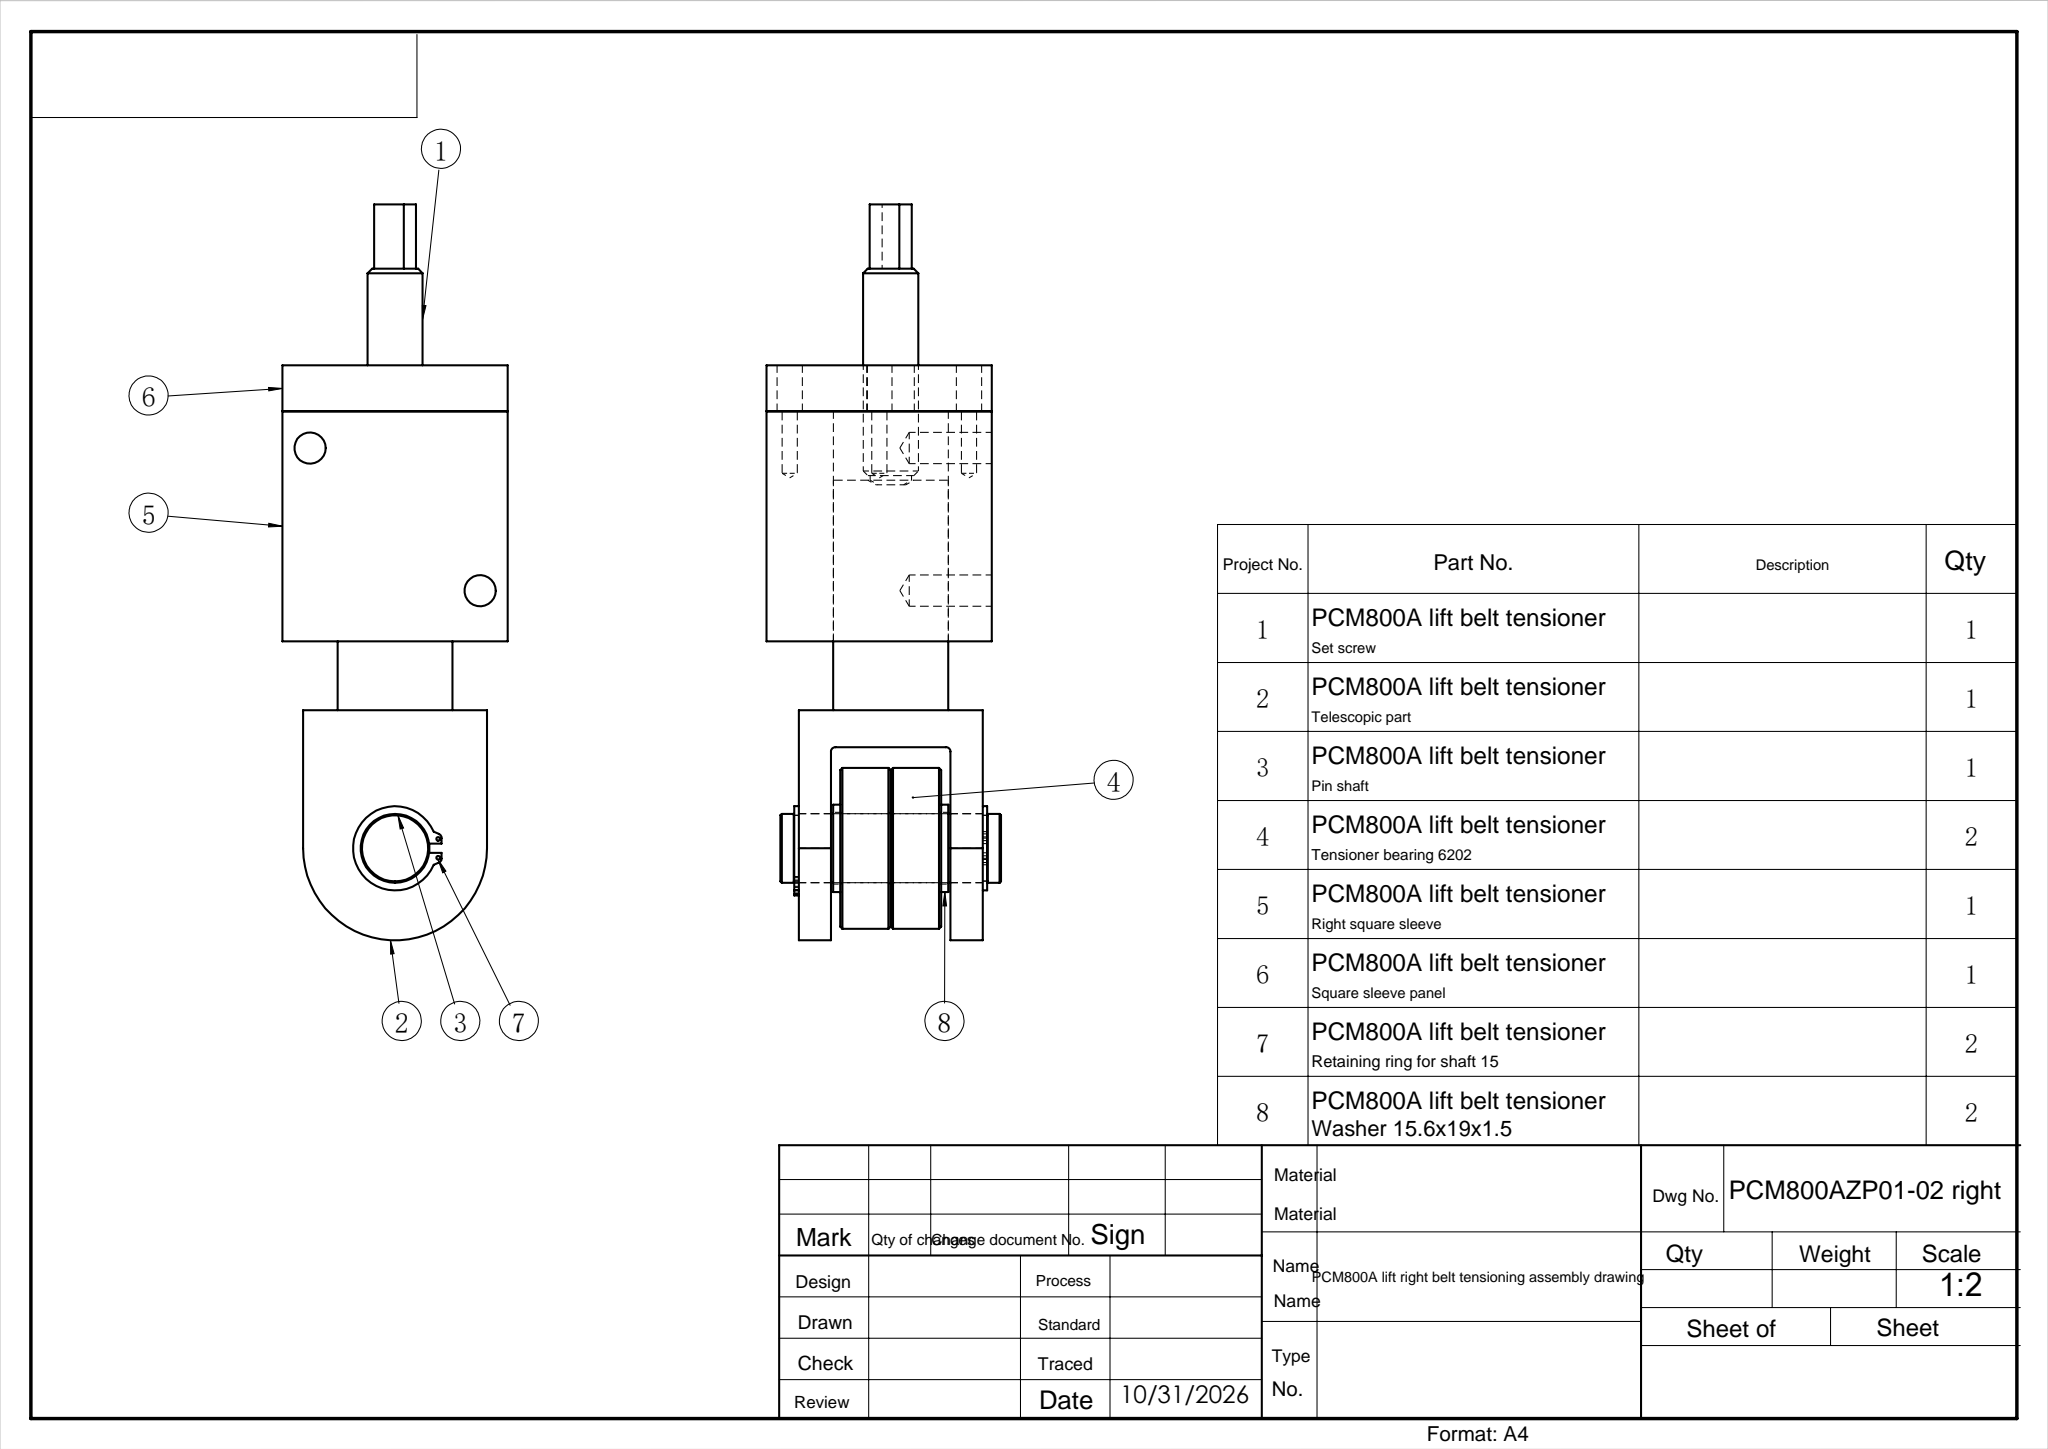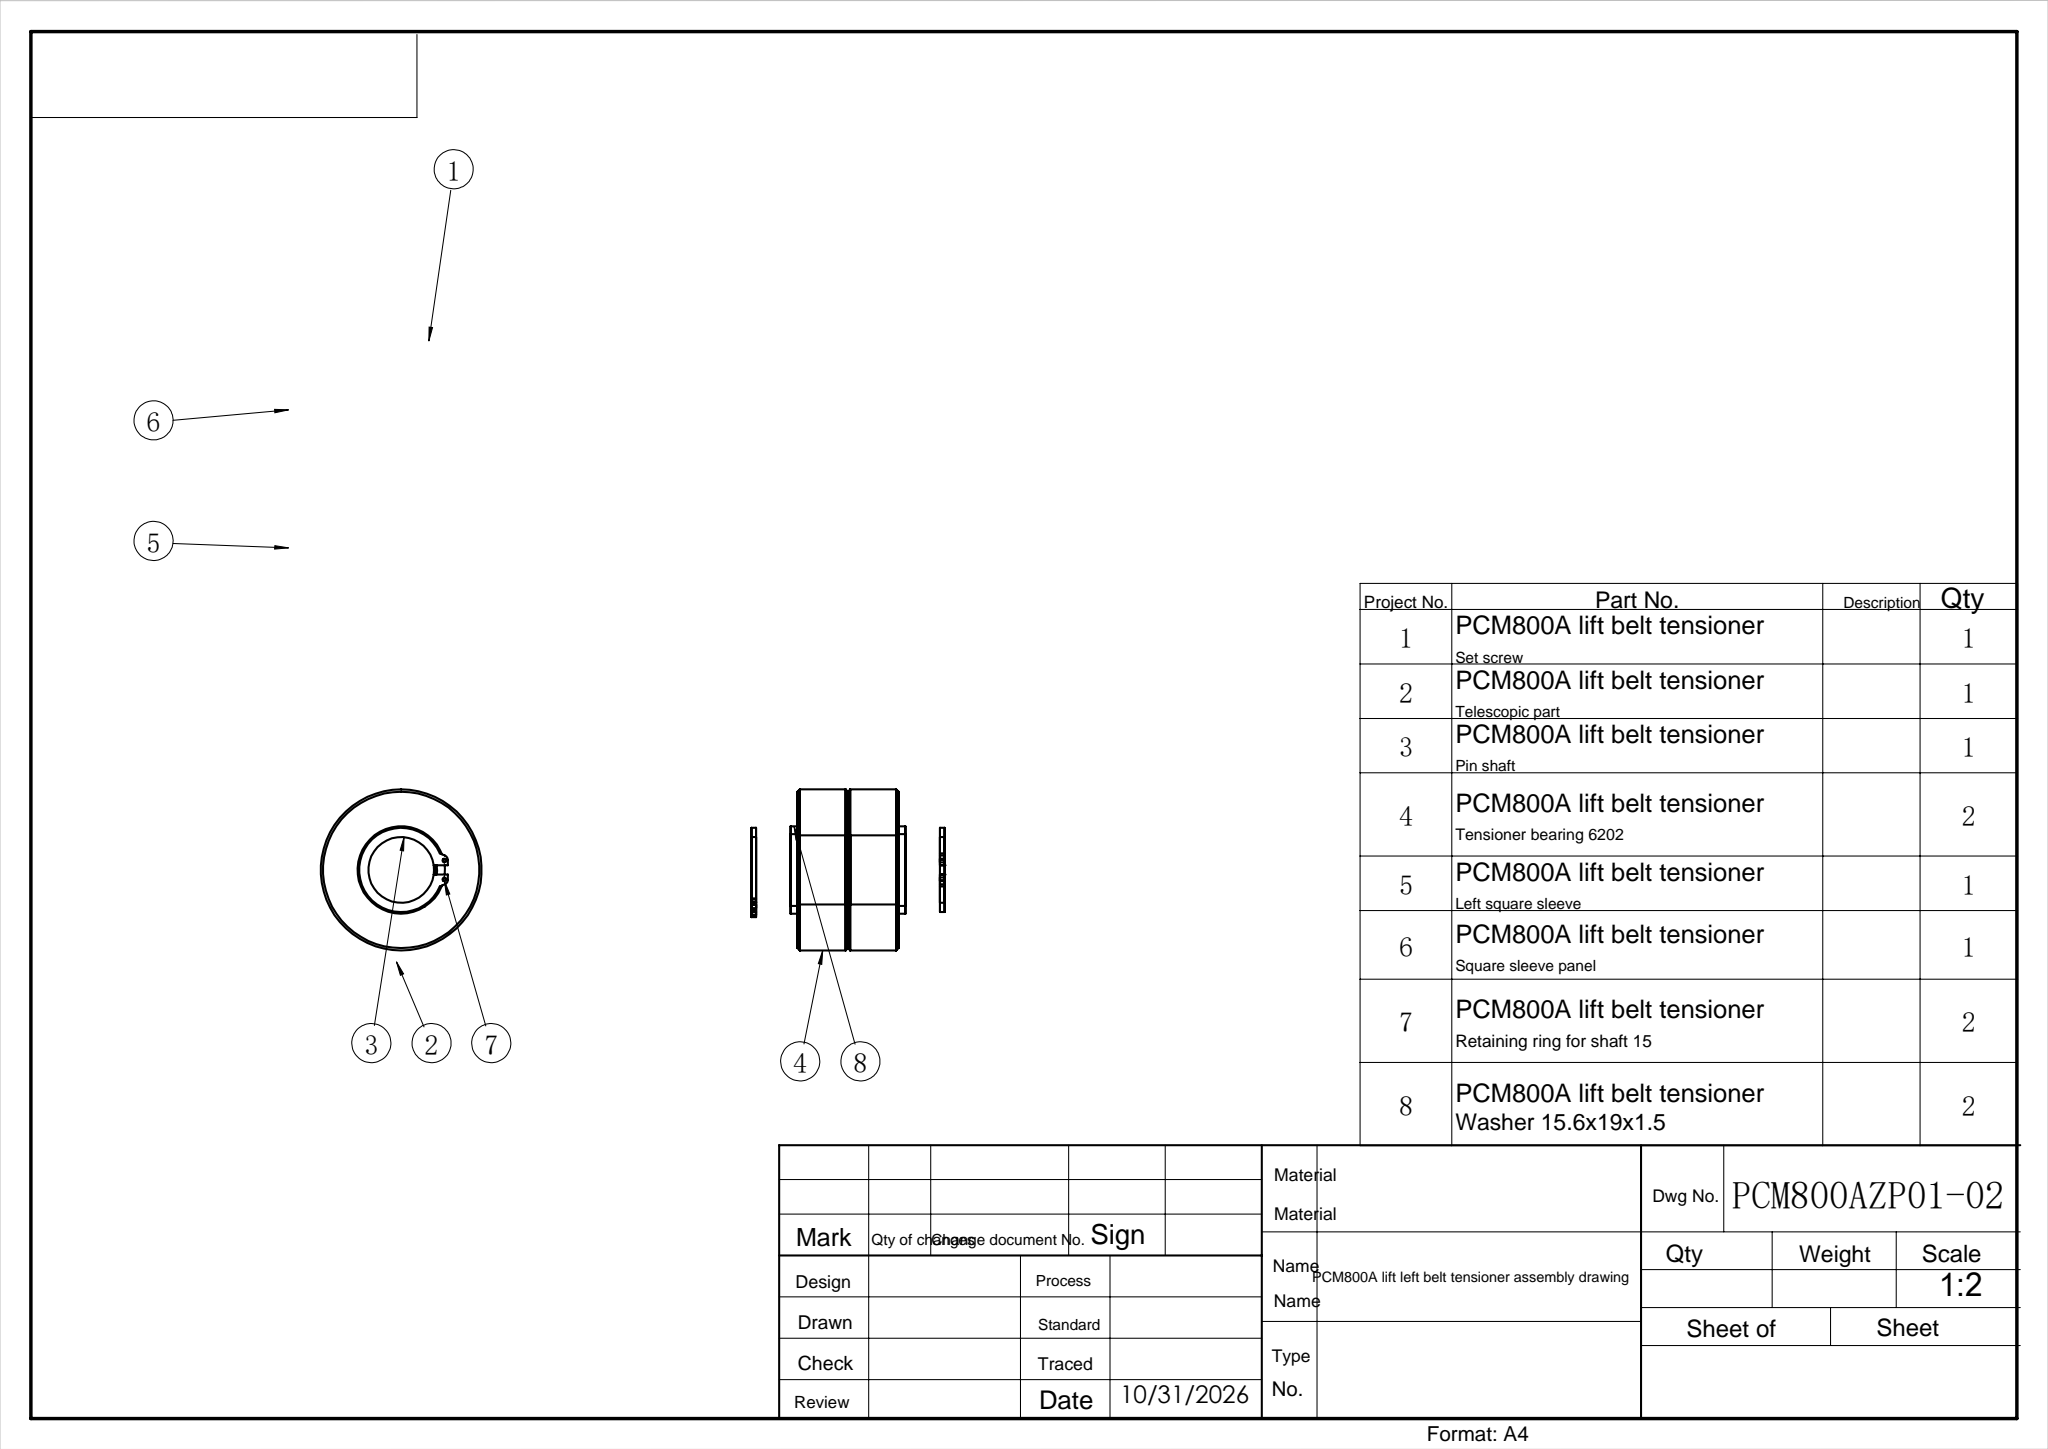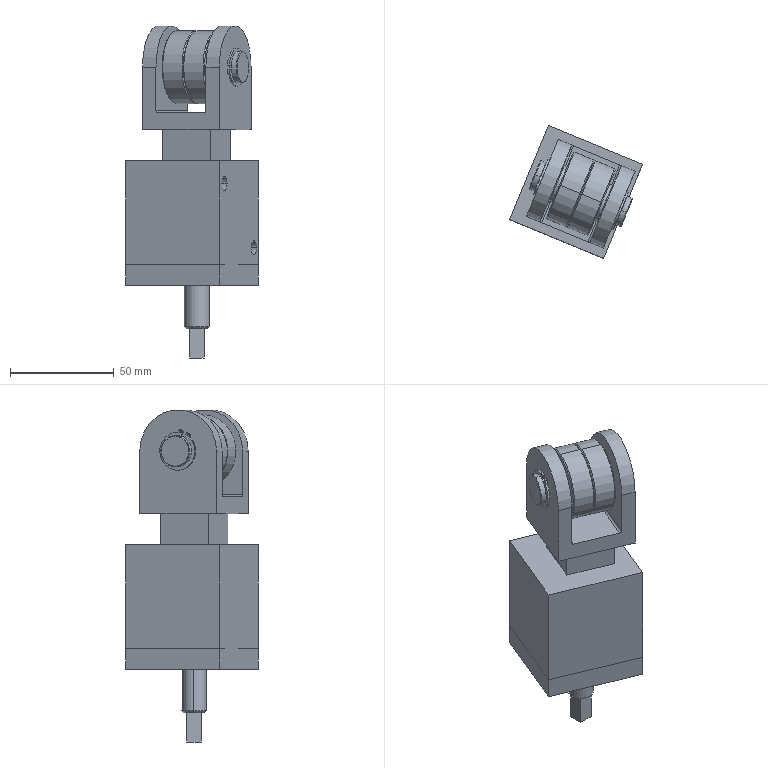Part | SolidWorks | 11 solids | 192 faces | box 64.002 x 64.002 x 160 mm | volume 203839 mm3 | cylinder 84 | plane 68 | cone 40 | commonest cylinder face diameters 15 x14 14.3 x10 0.8 x8 3.3 x8 5.5 x8 2 x6